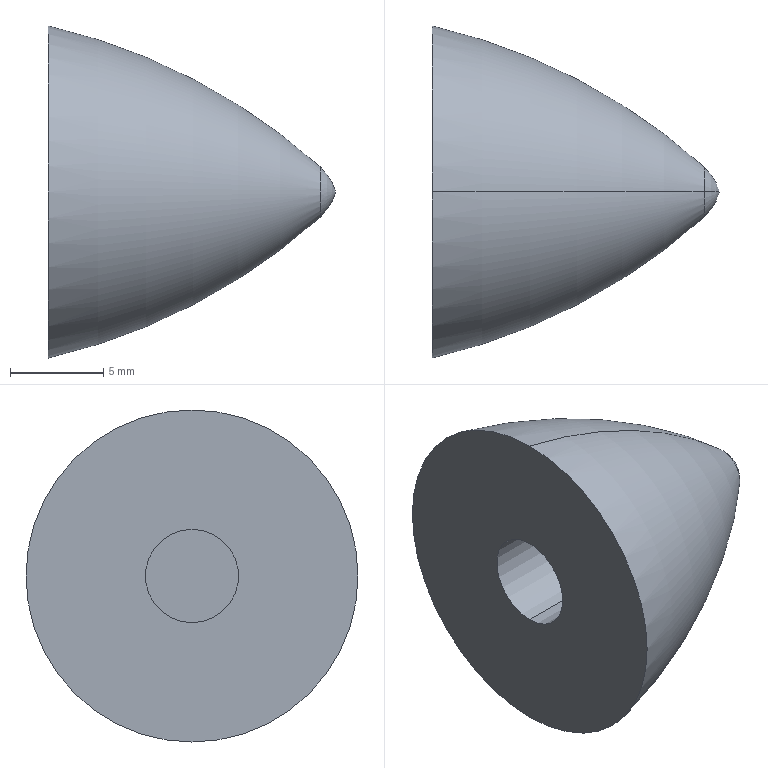Part | SolidWorks | features BaseBody 1 | 1 solid | 8 faces | box 15.4 x 17.8 x 17.8 mm | volume 1658 mm3 | torus 4 | plane 2 | cylinder 2 | commonest cylinder face diameters 5 x2
STEP:
#1=CARTESIAN_POINT('',(17.225,0.,0.));
#2=VERTEX_POINT('',#1);
#3=CARTESIAN_POINT('',(16.402,0.,1.346));
#4=VERTEX_POINT('',#3);
#5=CARTESIAN_POINT('',(14.345,0.,-0.8374));
#6=DIRECTION('',(0.,-1.,0.));
#7=DIRECTION('',(0.,0.,-1.));
#8=AXIS2_PLACEMENT_3D('',#5,#6,#7);
#9=CIRCLE('',#8,3.);
#10=EDGE_CURVE('',#2,#4,#9,.T.);
#11=ORIENTED_EDGE('',*,*,#10,.F.);
#12=CARTESIAN_POINT('',(16.402,0.,-1.346));
#13=VERTEX_POINT('',#12);
#14=CARTESIAN_POINT('',(14.345,0.,0.8374));
#15=DIRECTION('',(0.,1.,0.));
#16=DIRECTION('',(0.,0.,1.));
#17=AXIS2_PLACEMENT_3D('',#14,#15,#16);
#18=CIRCLE('',#17,3.);
#19=EDGE_CURVE('',#2,#13,#18,.T.);
#20=ORIENTED_EDGE('',*,*,#19,.T.);
#21=CARTESIAN_POINT('',(16.402,0.,0.));
#22=DIRECTION('',(-1.,0.,0.));
#23=DIRECTION('',(0.,0.,1.));
#24=AXIS2_PLACEMENT_3D('',#21,#22,#23);
#25=CIRCLE('',#24,1.346);
#26=EDGE_CURVE('',#4,#13,#25,.T.);
#27=ORIENTED_EDGE('',*,*,#26,.F.);
#28=EDGE_LOOP('',(#11,#20,#27));
#29=FACE_OUTER_BOUND('',#28,.T.);
#30=CARTESIAN_POINT('',(14.345,0.,0.));
#31=DIRECTION('',(-1.,0.,0.));
#32=DIRECTION('',(0.,0.,1.));
#33=AXIS2_PLACEMENT_3D('',#30,#31,#32);
#34=TOROIDAL_SURFACE('',#33,-0.8374,3.);
#35=ADVANCED_FACE('',(#29),#34,.T.);
#36=ORIENTED_EDGE('',*,*,#26,.T.);
#37=CARTESIAN_POINT('',(1.825,0.,-8.9));
#38=VERTEX_POINT('',#37);
#39=CARTESIAN_POINT('',(-5.593,0.,23.255));
#40=DIRECTION('',(0.,1.,0.));
#41=DIRECTION('',(0.,0.,1.));
#42=AXIS2_PLACEMENT_3D('',#39,#40,#41);
#43=CIRCLE('',#42,33.);
#44=EDGE_CURVE('',#13,#38,#43,.T.);
#45=ORIENTED_EDGE('',*,*,#44,.T.);
#46=CARTESIAN_POINT('',(1.825,0.,8.9));
#47=VERTEX_POINT('',#46);
#48=CARTESIAN_POINT('',(1.825,0.,0.));
#49=DIRECTION('',(-1.,0.,0.));
#50=DIRECTION('',(0.,0.,1.));
#51=AXIS2_PLACEMENT_3D('',#48,#49,#50);
#52=CIRCLE('',#51,8.9);
#53=EDGE_CURVE('',#47,#38,#52,.T.);
#54=ORIENTED_EDGE('',*,*,#53,.F.);
#55=CARTESIAN_POINT('',(-5.593,0.,-23.255));
#56=DIRECTION('',(0.,-1.,0.));
#57=DIRECTION('',(0.,0.,-1.));
#58=AXIS2_PLACEMENT_3D('',#55,#56,#57);
#59=CIRCLE('',#58,33.);
#60=EDGE_CURVE('',#4,#47,#59,.T.);
#61=ORIENTED_EDGE('',*,*,#60,.F.);
#62=EDGE_LOOP('',(#36,#45,#54,#61));
#63=FACE_OUTER_BOUND('',#62,.T.);
#64=CARTESIAN_POINT('',(-5.593,0.,0.));
#65=DIRECTION('',(-1.,0.,0.));
#66=DIRECTION('',(0.,0.,1.));
#67=AXIS2_PLACEMENT_3D('',#64,#65,#66);
#68=TOROIDAL_SURFACE('',#67,-23.255,33.);
#69=ADVANCED_FACE('',(#63),#68,.T.);
#70=CARTESIAN_POINT('',(9.825,0.,-2.5));
#71=VERTEX_POINT('',#70);
#72=CARTESIAN_POINT('',(9.825,0.,2.5));
#73=VERTEX_POINT('',#72);
#74=CARTESIAN_POINT('',(9.825,0.,0.));
#75=DIRECTION('',(-1.,0.,0.));
#76=DIRECTION('',(0.,0.,1.));
#77=AXIS2_PLACEMENT_3D('',#74,#75,#76);
#78=CIRCLE('',#77,2.5);
#79=EDGE_CURVE('',#71,#73,#78,.T.);
#80=ORIENTED_EDGE('',*,*,#79,.F.);
#81=CARTESIAN_POINT('',(1.825,0.,-2.5));
#82=VERTEX_POINT('',#81);
#83=CARTESIAN_POINT('',(9.825,0.,-2.5));
#84=DIRECTION('',(-1.,0.,0.));
#85=VECTOR('',#84,1000.);
#86=LINE('',#83,#85);
#87=EDGE_CURVE('',#71,#82,#86,.T.);
#88=ORIENTED_EDGE('',*,*,#87,.T.);
#89=CARTESIAN_POINT('',(1.825,0.,2.5));
#90=VERTEX_POINT('',#89);
#91=CARTESIAN_POINT('',(1.825,0.,0.));
#92=DIRECTION('',(-1.,0.,0.));
#93=DIRECTION('',(0.,0.,1.));
#94=AXIS2_PLACEMENT_3D('',#91,#92,#93);
#95=CIRCLE('',#94,2.5);
#96=EDGE_CURVE('',#82,#90,#95,.T.);
#97=ORIENTED_EDGE('',*,*,#96,.T.);
#98=CARTESIAN_POINT('',(9.825,0.,2.5));
#99=DIRECTION('',(-1.,0.,0.));
#100=VECTOR('',#99,1000.);
#101=LINE('',#98,#100);
#102=EDGE_CURVE('',#73,#90,#101,.T.);
#103=ORIENTED_EDGE('',*,*,#102,.F.);
#104=EDGE_LOOP('',(#80,#88,#97,#103));
#105=FACE_OUTER_BOUND('',#104,.T.);
#106=CARTESIAN_POINT('',(9.825,0.,0.));
#107=DIRECTION('',(-1.,0.,0.));
#108=DIRECTION('',(0.,0.,1.));
#109=AXIS2_PLACEMENT_3D('',#106,#107,#108);
#110=CYLINDRICAL_SURFACE('',#109,2.5);
#111=ADVANCED_FACE('',(#105),#110,.F.);
#112=CARTESIAN_POINT('',(9.825,0.,0.));
#113=DIRECTION('',(-1.,0.,0.));
#114=DIRECTION('',(0.,0.,1.));
#115=AXIS2_PLACEMENT_3D('',#112,#113,#114);
#116=CIRCLE('',#115,2.5);
#117=EDGE_CURVE('',#73,#71,#116,.T.);
#118=ORIENTED_EDGE('',*,*,#117,.T.);
#119=ORIENTED_EDGE('',*,*,#79,.T.);
#120=EDGE_LOOP('',(#118,#119));
#121=FACE_OUTER_BOUND('',#120,.T.);
#122=CARTESIAN_POINT('',(9.825,2.5,0.));
#123=DIRECTION('',(1.,0.,0.));
#124=DIRECTION('',(0.,0.,-1.));
#125=AXIS2_PLACEMENT_3D('',#122,#123,#124);
#126=PLANE('',#125);
#127=ADVANCED_FACE('',(#121),#126,.F.);
#128=ORIENTED_EDGE('',*,*,#87,.F.);
#129=ORIENTED_EDGE('',*,*,#117,.F.);
#130=ORIENTED_EDGE('',*,*,#102,.T.);
#131=CARTESIAN_POINT('',(1.825,0.,0.));
#132=DIRECTION('',(-1.,0.,0.));
#133=DIRECTION('',(0.,0.,1.));
#134=AXIS2_PLACEMENT_3D('',#131,#132,#133);
#135=CIRCLE('',#134,2.5);
#136=EDGE_CURVE('',#90,#82,#135,.T.);
#137=ORIENTED_EDGE('',*,*,#136,.T.);
#138=EDGE_LOOP('',(#128,#129,#130,#137));
#139=FACE_OUTER_BOUND('',#138,.T.);
#140=CARTESIAN_POINT('',(9.825,0.,0.));
#141=DIRECTION('',(-1.,0.,0.));
#142=DIRECTION('',(0.,0.,1.));
#143=AXIS2_PLACEMENT_3D('',#140,#141,#142);
#144=CYLINDRICAL_SURFACE('',#143,2.5);
#145=ADVANCED_FACE('',(#139),#144,.F.);
#146=ORIENTED_EDGE('',*,*,#136,.F.);
#147=ORIENTED_EDGE('',*,*,#96,.F.);
#148=EDGE_LOOP('',(#146,#147));
#149=FACE_BOUND('',#148,.T.);
#150=ORIENTED_EDGE('',*,*,#53,.T.);
#151=CARTESIAN_POINT('',(1.825,0.,0.));
#152=DIRECTION('',(-1.,0.,0.));
#153=DIRECTION('',(0.,0.,1.));
#154=AXIS2_PLACEMENT_3D('',#151,#152,#153);
#155=CIRCLE('',#154,8.9);
#156=EDGE_CURVE('',#38,#47,#155,.T.);
#157=ORIENTED_EDGE('',*,*,#156,.T.);
#158=EDGE_LOOP('',(#150,#157));
#159=FACE_OUTER_BOUND('',#158,.T.);
#160=CARTESIAN_POINT('',(1.825,2.5,0.));
#161=DIRECTION('',(1.,0.,0.));
#162=DIRECTION('',(0.,0.,-1.));
#163=AXIS2_PLACEMENT_3D('',#160,#161,#162);
#164=PLANE('',#163);
#165=ADVANCED_FACE('',(#149,#159),#164,.F.);
#166=ORIENTED_EDGE('',*,*,#44,.F.);
#167=CARTESIAN_POINT('',(16.402,0.,0.));
#168=DIRECTION('',(-1.,0.,0.));
#169=DIRECTION('',(0.,0.,1.));
#170=AXIS2_PLACEMENT_3D('',#167,#168,#169);
#171=CIRCLE('',#170,1.346);
#172=EDGE_CURVE('',#13,#4,#171,.T.);
#173=ORIENTED_EDGE('',*,*,#172,.T.);
#174=ORIENTED_EDGE('',*,*,#60,.T.);
#175=ORIENTED_EDGE('',*,*,#156,.F.);
#176=EDGE_LOOP('',(#166,#173,#174,#175));
#177=FACE_OUTER_BOUND('',#176,.T.);
#178=CARTESIAN_POINT('',(-5.593,0.,0.));
#179=DIRECTION('',(-1.,0.,0.));
#180=DIRECTION('',(0.,0.,1.));
#181=AXIS2_PLACEMENT_3D('',#178,#179,#180);
#182=TOROIDAL_SURFACE('',#181,-23.255,33.);
#183=ADVANCED_FACE('',(#177),#182,.T.);
#184=ORIENTED_EDGE('',*,*,#19,.F.);
#185=ORIENTED_EDGE('',*,*,#10,.T.);
#186=ORIENTED_EDGE('',*,*,#172,.F.);
#187=EDGE_LOOP('',(#184,#185,#186));
#188=FACE_OUTER_BOUND('',#187,.T.);
#189=CARTESIAN_POINT('',(14.345,0.,0.));
#190=DIRECTION('',(-1.,0.,0.));
#191=DIRECTION('',(0.,0.,1.));
#192=AXIS2_PLACEMENT_3D('',#189,#190,#191);
#193=TOROIDAL_SURFACE('',#192,-0.8374,3.);
#194=ADVANCED_FACE('',(#188),#193,.T.);
#195=CLOSED_SHELL('',(#35,#69,#111,#127,#145,#165,#183,#194));
#196=MANIFOLD_SOLID_BREP('',#195);
#197=CARTESIAN_POINT('',(0.,0.,0.));
#198=DIRECTION('',(0.,0.,1.));
#199=DIRECTION('',(1.,0.,0.));
#200=AXIS2_PLACEMENT_3D('',#197,#198,#199);
#201=(LENGTH_UNIT()NAMED_UNIT(*)SI_UNIT(.MILLI.,.METRE.));
#202=UNCERTAINTY_MEASURE_WITH_UNIT(LENGTH_MEASURE(0.00001),#201,'','');
#203=(NAMED_UNIT(*)PLANE_ANGLE_UNIT()SI_UNIT($,.RADIAN.));
#204=(NAMED_UNIT(*)SI_UNIT($,.STERADIAN.)SOLID_ANGLE_UNIT());
#205=(GEOMETRIC_REPRESENTATION_CONTEXT(3)GLOBAL_UNCERTAINTY_ASSIGNED_CONTEXT((#202))GLOBAL_UNIT_ASSIGNED_CONTEXT((#201,#203,#204))REPRESENTATION_CONTEXT('',''));
#206=ADVANCED_BREP_SHAPE_REPRESENTATION('',(#196,#200),#205);